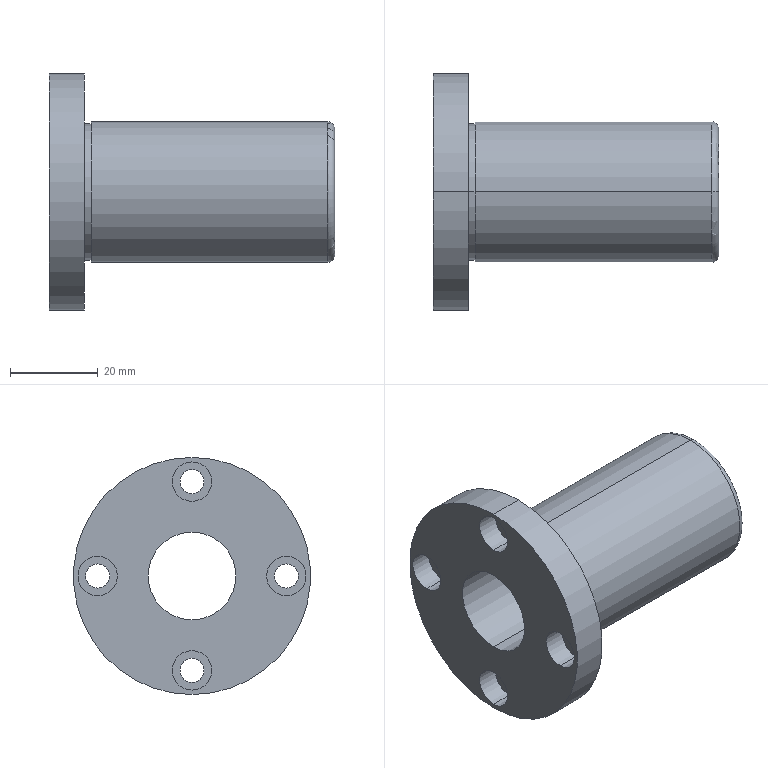Part | SolidWorks | features LPattern 1, RevCut 1, Revolution 1 | 1 solid | 34 faces | box 65 x 54 x 54 mm | volume 42042 mm3 | cylinder 24 | plane 8 | torus 2 | commonest cylinder face diameters 5.5 x8 9 x8 20 x2 31 x2 32 x2 54 x2
STEP:
#1=CARTESIAN_POINT('',(8.,-21.5,-2.75));
#2=VERTEX_POINT('',#1);
#3=CARTESIAN_POINT('',(8.,-21.5,2.75));
#4=VERTEX_POINT('',#3);
#5=CARTESIAN_POINT('',(8.,-21.5,0.));
#6=DIRECTION('',(-1.,0.,0.));
#7=DIRECTION('',(0.,0.,1.));
#8=AXIS2_PLACEMENT_3D('',#5,#6,#7);
#9=CIRCLE('',#8,2.75);
#10=EDGE_CURVE('',#2,#4,#9,.T.);
#11=ORIENTED_EDGE('',*,*,#10,.F.);
#12=CARTESIAN_POINT('',(5.1,-21.5,-2.75));
#13=VERTEX_POINT('',#12);
#14=CARTESIAN_POINT('',(8.,-21.5,-2.75));
#15=DIRECTION('',(-1.,0.,0.));
#16=VECTOR('',#15,1000.);
#17=LINE('',#14,#16);
#18=EDGE_CURVE('',#2,#13,#17,.T.);
#19=ORIENTED_EDGE('',*,*,#18,.T.);
#20=CARTESIAN_POINT('',(5.1,-21.5,2.75));
#21=VERTEX_POINT('',#20);
#22=CARTESIAN_POINT('',(5.1,-21.5,0.));
#23=DIRECTION('',(-1.,0.,0.));
#24=DIRECTION('',(0.,0.,1.));
#25=AXIS2_PLACEMENT_3D('',#22,#23,#24);
#26=CIRCLE('',#25,2.75);
#27=EDGE_CURVE('',#13,#21,#26,.T.);
#28=ORIENTED_EDGE('',*,*,#27,.T.);
#29=CARTESIAN_POINT('',(8.,-21.5,2.75));
#30=DIRECTION('',(-1.,0.,0.));
#31=VECTOR('',#30,1000.);
#32=LINE('',#29,#31);
#33=EDGE_CURVE('',#4,#21,#32,.T.);
#34=ORIENTED_EDGE('',*,*,#33,.F.);
#35=EDGE_LOOP('',(#11,#19,#28,#34));
#36=FACE_OUTER_BOUND('',#35,.T.);
#37=CARTESIAN_POINT('',(8.,-21.5,0.));
#38=DIRECTION('',(-1.,0.,0.));
#39=DIRECTION('',(0.,0.,1.));
#40=AXIS2_PLACEMENT_3D('',#37,#38,#39);
#41=CYLINDRICAL_SURFACE('',#40,2.75);
#42=ADVANCED_FACE('',(#36),#41,.F.);
#43=CARTESIAN_POINT('',(5.1,-21.5,-4.5));
#44=VERTEX_POINT('',#43);
#45=CARTESIAN_POINT('',(5.1,-21.5,4.5));
#46=VERTEX_POINT('',#45);
#47=CARTESIAN_POINT('',(5.1,-21.5,0.));
#48=DIRECTION('',(-1.,0.,0.));
#49=DIRECTION('',(0.,0.,1.));
#50=AXIS2_PLACEMENT_3D('',#47,#48,#49);
#51=CIRCLE('',#50,4.5);
#52=EDGE_CURVE('',#44,#46,#51,.T.);
#53=ORIENTED_EDGE('',*,*,#52,.F.);
#54=CARTESIAN_POINT('',(0.,-21.5,-4.5));
#55=VERTEX_POINT('',#54);
#56=CARTESIAN_POINT('',(8.,-21.5,-4.5));
#57=DIRECTION('',(-1.,0.,0.));
#58=VECTOR('',#57,1000.);
#59=LINE('',#56,#58);
#60=EDGE_CURVE('',#44,#55,#59,.T.);
#61=ORIENTED_EDGE('',*,*,#60,.T.);
#62=CARTESIAN_POINT('',(0.,-21.5,4.5));
#63=VERTEX_POINT('',#62);
#64=CARTESIAN_POINT('',(0.,-21.5,0.));
#65=DIRECTION('',(-1.,0.,0.));
#66=DIRECTION('',(0.,0.,1.));
#67=AXIS2_PLACEMENT_3D('',#64,#65,#66);
#68=CIRCLE('',#67,4.5);
#69=EDGE_CURVE('',#55,#63,#68,.T.);
#70=ORIENTED_EDGE('',*,*,#69,.T.);
#71=CARTESIAN_POINT('',(8.,-21.5,4.5));
#72=DIRECTION('',(-1.,0.,0.));
#73=VECTOR('',#72,1000.);
#74=LINE('',#71,#73);
#75=EDGE_CURVE('',#46,#63,#74,.T.);
#76=ORIENTED_EDGE('',*,*,#75,.F.);
#77=EDGE_LOOP('',(#53,#61,#70,#76));
#78=FACE_OUTER_BOUND('',#77,.T.);
#79=CARTESIAN_POINT('',(8.,-21.5,0.));
#80=DIRECTION('',(-1.,0.,0.));
#81=DIRECTION('',(0.,0.,1.));
#82=AXIS2_PLACEMENT_3D('',#79,#80,#81);
#83=CYLINDRICAL_SURFACE('',#82,4.5);
#84=ADVANCED_FACE('',(#78),#83,.F.);
#85=CARTESIAN_POINT('',(8.,0.,18.75));
#86=VERTEX_POINT('',#85);
#87=CARTESIAN_POINT('',(8.,0.,24.25));
#88=VERTEX_POINT('',#87);
#89=CARTESIAN_POINT('',(8.,0.,21.5));
#90=DIRECTION('',(-1.,0.,0.));
#91=DIRECTION('',(0.,0.,1.));
#92=AXIS2_PLACEMENT_3D('',#89,#90,#91);
#93=CIRCLE('',#92,2.75);
#94=EDGE_CURVE('',#86,#88,#93,.T.);
#95=ORIENTED_EDGE('',*,*,#94,.F.);
#96=CARTESIAN_POINT('',(5.1,0.,18.75));
#97=VERTEX_POINT('',#96);
#98=CARTESIAN_POINT('',(8.,0.,18.75));
#99=DIRECTION('',(-1.,0.,0.));
#100=VECTOR('',#99,1000.);
#101=LINE('',#98,#100);
#102=EDGE_CURVE('',#86,#97,#101,.T.);
#103=ORIENTED_EDGE('',*,*,#102,.T.);
#104=CARTESIAN_POINT('',(5.1,0.,24.25));
#105=VERTEX_POINT('',#104);
#106=CARTESIAN_POINT('',(5.1,0.,21.5));
#107=DIRECTION('',(-1.,0.,0.));
#108=DIRECTION('',(0.,0.,1.));
#109=AXIS2_PLACEMENT_3D('',#106,#107,#108);
#110=CIRCLE('',#109,2.75);
#111=EDGE_CURVE('',#97,#105,#110,.T.);
#112=ORIENTED_EDGE('',*,*,#111,.T.);
#113=CARTESIAN_POINT('',(8.,0.,24.25));
#114=DIRECTION('',(-1.,0.,0.));
#115=VECTOR('',#114,1000.);
#116=LINE('',#113,#115);
#117=EDGE_CURVE('',#88,#105,#116,.T.);
#118=ORIENTED_EDGE('',*,*,#117,.F.);
#119=EDGE_LOOP('',(#95,#103,#112,#118));
#120=FACE_OUTER_BOUND('',#119,.T.);
#121=CARTESIAN_POINT('',(8.,0.,21.5));
#122=DIRECTION('',(-1.,0.,0.));
#123=DIRECTION('',(0.,0.,1.));
#124=AXIS2_PLACEMENT_3D('',#121,#122,#123);
#125=CYLINDRICAL_SURFACE('',#124,2.75);
#126=ADVANCED_FACE('',(#120),#125,.F.);
#127=CARTESIAN_POINT('',(5.1,0.,17.));
#128=VERTEX_POINT('',#127);
#129=CARTESIAN_POINT('',(5.1,0.,26.));
#130=VERTEX_POINT('',#129);
#131=CARTESIAN_POINT('',(5.1,0.,21.5));
#132=DIRECTION('',(-1.,0.,0.));
#133=DIRECTION('',(0.,0.,1.));
#134=AXIS2_PLACEMENT_3D('',#131,#132,#133);
#135=CIRCLE('',#134,4.5);
#136=EDGE_CURVE('',#128,#130,#135,.T.);
#137=ORIENTED_EDGE('',*,*,#136,.F.);
#138=CARTESIAN_POINT('',(0.,0.,17.));
#139=VERTEX_POINT('',#138);
#140=CARTESIAN_POINT('',(8.,0.,17.));
#141=DIRECTION('',(-1.,0.,0.));
#142=VECTOR('',#141,1000.);
#143=LINE('',#140,#142);
#144=EDGE_CURVE('',#128,#139,#143,.T.);
#145=ORIENTED_EDGE('',*,*,#144,.T.);
#146=CARTESIAN_POINT('',(0.,0.,26.));
#147=VERTEX_POINT('',#146);
#148=CARTESIAN_POINT('',(0.,0.,21.5));
#149=DIRECTION('',(-1.,0.,0.));
#150=DIRECTION('',(0.,0.,1.));
#151=AXIS2_PLACEMENT_3D('',#148,#149,#150);
#152=CIRCLE('',#151,4.5);
#153=EDGE_CURVE('',#139,#147,#152,.T.);
#154=ORIENTED_EDGE('',*,*,#153,.T.);
#155=CARTESIAN_POINT('',(8.,0.,26.));
#156=DIRECTION('',(-1.,0.,0.));
#157=VECTOR('',#156,1000.);
#158=LINE('',#155,#157);
#159=EDGE_CURVE('',#130,#147,#158,.T.);
#160=ORIENTED_EDGE('',*,*,#159,.F.);
#161=EDGE_LOOP('',(#137,#145,#154,#160));
#162=FACE_OUTER_BOUND('',#161,.T.);
#163=CARTESIAN_POINT('',(8.,0.,21.5));
#164=DIRECTION('',(-1.,0.,0.));
#165=DIRECTION('',(0.,0.,1.));
#166=AXIS2_PLACEMENT_3D('',#163,#164,#165);
#167=CYLINDRICAL_SURFACE('',#166,4.5);
#168=ADVANCED_FACE('',(#162),#167,.F.);
#169=CARTESIAN_POINT('',(8.,0.,-24.25));
#170=VERTEX_POINT('',#169);
#171=CARTESIAN_POINT('',(8.,0.,-18.75));
#172=VERTEX_POINT('',#171);
#173=CARTESIAN_POINT('',(8.,0.,-21.5));
#174=DIRECTION('',(-1.,0.,0.));
#175=DIRECTION('',(0.,0.,1.));
#176=AXIS2_PLACEMENT_3D('',#173,#174,#175);
#177=CIRCLE('',#176,2.75);
#178=EDGE_CURVE('',#170,#172,#177,.T.);
#179=ORIENTED_EDGE('',*,*,#178,.F.);
#180=CARTESIAN_POINT('',(5.1,0.,-24.25));
#181=VERTEX_POINT('',#180);
#182=CARTESIAN_POINT('',(8.,0.,-24.25));
#183=DIRECTION('',(-1.,0.,0.));
#184=VECTOR('',#183,1000.);
#185=LINE('',#182,#184);
#186=EDGE_CURVE('',#170,#181,#185,.T.);
#187=ORIENTED_EDGE('',*,*,#186,.T.);
#188=CARTESIAN_POINT('',(5.1,0.,-18.75));
#189=VERTEX_POINT('',#188);
#190=CARTESIAN_POINT('',(5.1,0.,-21.5));
#191=DIRECTION('',(-1.,0.,0.));
#192=DIRECTION('',(0.,0.,1.));
#193=AXIS2_PLACEMENT_3D('',#190,#191,#192);
#194=CIRCLE('',#193,2.75);
#195=EDGE_CURVE('',#181,#189,#194,.T.);
#196=ORIENTED_EDGE('',*,*,#195,.T.);
#197=CARTESIAN_POINT('',(8.,0.,-18.75));
#198=DIRECTION('',(-1.,0.,0.));
#199=VECTOR('',#198,1000.);
#200=LINE('',#197,#199);
#201=EDGE_CURVE('',#172,#189,#200,.T.);
#202=ORIENTED_EDGE('',*,*,#201,.F.);
#203=EDGE_LOOP('',(#179,#187,#196,#202));
#204=FACE_OUTER_BOUND('',#203,.T.);
#205=CARTESIAN_POINT('',(8.,0.,-21.5));
#206=DIRECTION('',(-1.,0.,0.));
#207=DIRECTION('',(0.,0.,1.));
#208=AXIS2_PLACEMENT_3D('',#205,#206,#207);
#209=CYLINDRICAL_SURFACE('',#208,2.75);
#210=ADVANCED_FACE('',(#204),#209,.F.);
#211=CARTESIAN_POINT('',(5.1,0.,-26.));
#212=VERTEX_POINT('',#211);
#213=CARTESIAN_POINT('',(5.1,0.,-17.));
#214=VERTEX_POINT('',#213);
#215=CARTESIAN_POINT('',(5.1,0.,-21.5));
#216=DIRECTION('',(-1.,0.,0.));
#217=DIRECTION('',(0.,0.,1.));
#218=AXIS2_PLACEMENT_3D('',#215,#216,#217);
#219=CIRCLE('',#218,4.5);
#220=EDGE_CURVE('',#212,#214,#219,.T.);
#221=ORIENTED_EDGE('',*,*,#220,.F.);
#222=CARTESIAN_POINT('',(0.,0.,-26.));
#223=VERTEX_POINT('',#222);
#224=CARTESIAN_POINT('',(8.,0.,-26.));
#225=DIRECTION('',(-1.,0.,0.));
#226=VECTOR('',#225,1000.);
#227=LINE('',#224,#226);
#228=EDGE_CURVE('',#212,#223,#227,.T.);
#229=ORIENTED_EDGE('',*,*,#228,.T.);
#230=CARTESIAN_POINT('',(0.,0.,-17.));
#231=VERTEX_POINT('',#230);
#232=CARTESIAN_POINT('',(0.,0.,-21.5));
#233=DIRECTION('',(-1.,0.,0.));
#234=DIRECTION('',(0.,0.,1.));
#235=AXIS2_PLACEMENT_3D('',#232,#233,#234);
#236=CIRCLE('',#235,4.5);
#237=EDGE_CURVE('',#223,#231,#236,.T.);
#238=ORIENTED_EDGE('',*,*,#237,.T.);
#239=CARTESIAN_POINT('',(8.,0.,-17.));
#240=DIRECTION('',(-1.,0.,0.));
#241=VECTOR('',#240,1000.);
#242=LINE('',#239,#241);
#243=EDGE_CURVE('',#214,#231,#242,.T.);
#244=ORIENTED_EDGE('',*,*,#243,.F.);
#245=EDGE_LOOP('',(#221,#229,#238,#244));
#246=FACE_OUTER_BOUND('',#245,.T.);
#247=CARTESIAN_POINT('',(8.,0.,-21.5));
#248=DIRECTION('',(-1.,0.,0.));
#249=DIRECTION('',(0.,0.,1.));
#250=AXIS2_PLACEMENT_3D('',#247,#248,#249);
#251=CYLINDRICAL_SURFACE('',#250,4.5);
#252=ADVANCED_FACE('',(#246),#251,.F.);
#253=CARTESIAN_POINT('',(8.,21.5,-2.75));
#254=VERTEX_POINT('',#253);
#255=CARTESIAN_POINT('',(8.,21.5,2.75));
#256=VERTEX_POINT('',#255);
#257=CARTESIAN_POINT('',(8.,21.5,0.));
#258=DIRECTION('',(-1.,0.,0.));
#259=DIRECTION('',(0.,0.,1.));
#260=AXIS2_PLACEMENT_3D('',#257,#258,#259);
#261=CIRCLE('',#260,2.75);
#262=EDGE_CURVE('',#254,#256,#261,.T.);
#263=ORIENTED_EDGE('',*,*,#262,.F.);
#264=CARTESIAN_POINT('',(5.1,21.5,-2.75));
#265=VERTEX_POINT('',#264);
#266=CARTESIAN_POINT('',(8.,21.5,-2.75));
#267=DIRECTION('',(-1.,0.,0.));
#268=VECTOR('',#267,1000.);
#269=LINE('',#266,#268);
#270=EDGE_CURVE('',#254,#265,#269,.T.);
#271=ORIENTED_EDGE('',*,*,#270,.T.);
#272=CARTESIAN_POINT('',(5.1,21.5,2.75));
#273=VERTEX_POINT('',#272);
#274=CARTESIAN_POINT('',(5.1,21.5,0.));
#275=DIRECTION('',(-1.,0.,0.));
#276=DIRECTION('',(0.,0.,1.));
#277=AXIS2_PLACEMENT_3D('',#274,#275,#276);
#278=CIRCLE('',#277,2.75);
#279=EDGE_CURVE('',#265,#273,#278,.T.);
#280=ORIENTED_EDGE('',*,*,#279,.T.);
#281=CARTESIAN_POINT('',(8.,21.5,2.75));
#282=DIRECTION('',(-1.,0.,0.));
#283=VECTOR('',#282,1000.);
#284=LINE('',#281,#283);
#285=EDGE_CURVE('',#256,#273,#284,.T.);
#286=ORIENTED_EDGE('',*,*,#285,.F.);
#287=EDGE_LOOP('',(#263,#271,#280,#286));
#288=FACE_OUTER_BOUND('',#287,.T.);
#289=CARTESIAN_POINT('',(8.,21.5,0.));
#290=DIRECTION('',(-1.,0.,0.));
#291=DIRECTION('',(0.,0.,1.));
#292=AXIS2_PLACEMENT_3D('',#289,#290,#291);
#293=CYLINDRICAL_SURFACE('',#292,2.75);
#294=ADVANCED_FACE('',(#288),#293,.F.);
#295=CARTESIAN_POINT('',(5.1,21.5,-4.5));
#296=VERTEX_POINT('',#295);
#297=CARTESIAN_POINT('',(5.1,21.5,4.5));
#298=VERTEX_POINT('',#297);
#299=CARTESIAN_POINT('',(5.1,21.5,0.));
#300=DIRECTION('',(-1.,0.,0.));
#301=DIRECTION('',(0.,0.,1.));
#302=AXIS2_PLACEMENT_3D('',#299,#300,#301);
#303=CIRCLE('',#302,4.5);
#304=EDGE_CURVE('',#296,#298,#303,.T.);
#305=ORIENTED_EDGE('',*,*,#304,.F.);
#306=CARTESIAN_POINT('',(0.,21.5,-4.5));
#307=VERTEX_POINT('',#306);
#308=CARTESIAN_POINT('',(8.,21.5,-4.5));
#309=DIRECTION('',(-1.,0.,0.));
#310=VECTOR('',#309,1000.);
#311=LINE('',#308,#310);
#312=EDGE_CURVE('',#296,#307,#311,.T.);
#313=ORIENTED_EDGE('',*,*,#312,.T.);
#314=CARTESIAN_POINT('',(0.,21.5,4.5));
#315=VERTEX_POINT('',#314);
#316=CARTESIAN_POINT('',(0.,21.5,0.));
#317=DIRECTION('',(-1.,0.,0.));
#318=DIRECTION('',(0.,0.,1.));
#319=AXIS2_PLACEMENT_3D('',#316,#317,#318);
#320=CIRCLE('',#319,4.5);
#321=EDGE_CURVE('',#307,#315,#320,.T.);
#322=ORIENTED_EDGE('',*,*,#321,.T.);
#323=CARTESIAN_POINT('',(8.,21.5,4.5));
#324=DIRECTION('',(-1.,0.,0.));
#325=VECTOR('',#324,1000.);
#326=LINE('',#323,#325);
#327=EDGE_CURVE('',#298,#315,#326,.T.);
#328=ORIENTED_EDGE('',*,*,#327,.F.);
#329=EDGE_LOOP('',(#305,#313,#322,#328));
#330=FACE_OUTER_BOUND('',#329,.T.);
#331=CARTESIAN_POINT('',(8.,21.5,0.));
#332=DIRECTION('',(-1.,0.,0.));
#333=DIRECTION('',(0.,0.,1.));
#334=AXIS2_PLACEMENT_3D('',#331,#332,#333);
#335=CYLINDRICAL_SURFACE('',#334,4.5);
#336=ADVANCED_FACE('',(#330),#335,.F.);
#337=CARTESIAN_POINT('',(9.5,0.,15.5));
#338=VERTEX_POINT('',#337);
#339=CARTESIAN_POINT('',(9.5,0.,-15.5));
#340=VERTEX_POINT('',#339);
#341=CARTESIAN_POINT('',(9.5,0.,0.));
#342=DIRECTION('',(-1.,0.,0.));
#343=DIRECTION('',(0.,0.,1.));
#344=AXIS2_PLACEMENT_3D('',#341,#342,#343);
#345=CIRCLE('',#344,15.5);
#346=EDGE_CURVE('',#338,#340,#345,.T.);
#347=ORIENTED_EDGE('',*,*,#346,.T.);
#348=CARTESIAN_POINT('',(8.,0.,-15.5));
#349=VERTEX_POINT('',#348);
#350=CARTESIAN_POINT('',(65.,0.,-15.5));
#351=DIRECTION('',(-1.,0.,0.));
#352=VECTOR('',#351,1000.);
#353=LINE('',#350,#352);
#354=EDGE_CURVE('',#340,#349,#353,.T.);
#355=ORIENTED_EDGE('',*,*,#354,.T.);
#356=CARTESIAN_POINT('',(8.,0.,15.5));
#357=VERTEX_POINT('',#356);
#358=CARTESIAN_POINT('',(8.,0.,0.));
#359=DIRECTION('',(-1.,0.,0.));
#360=DIRECTION('',(0.,0.,1.));
#361=AXIS2_PLACEMENT_3D('',#358,#359,#360);
#362=CIRCLE('',#361,15.5);
#363=EDGE_CURVE('',#357,#349,#362,.T.);
#364=ORIENTED_EDGE('',*,*,#363,.F.);
#365=CARTESIAN_POINT('',(65.,0.,15.5));
#366=DIRECTION('',(-1.,0.,0.));
#367=VECTOR('',#366,1000.);
#368=LINE('',#365,#367);
#369=EDGE_CURVE('',#338,#357,#368,.T.);
#370=ORIENTED_EDGE('',*,*,#369,.F.);
#371=EDGE_LOOP('',(#347,#355,#364,#370));
#372=FACE_OUTER_BOUND('',#371,.T.);
#373=CARTESIAN_POINT('',(65.,0.,0.));
#374=DIRECTION('',(-1.,0.,0.));
#375=DIRECTION('',(0.,0.,1.));
#376=AXIS2_PLACEMENT_3D('',#373,#374,#375);
#377=CYLINDRICAL_SURFACE('',#376,15.5);
#378=ADVANCED_FACE('',(#372),#377,.T.);
#379=CARTESIAN_POINT('',(63.4,0.,16.));
#380=VERTEX_POINT('',#379);
#381=CARTESIAN_POINT('',(63.4,0.,-16.));
#382=VERTEX_POINT('',#381);
#383=CARTESIAN_POINT('',(63.4,0.,0.));
#384=DIRECTION('',(-1.,0.,0.));
#385=DIRECTION('',(0.,0.,1.));
#386=AXIS2_PLACEMENT_3D('',#383,#384,#385);
#387=CIRCLE('',#386,16.);
#388=EDGE_CURVE('',#380,#382,#387,.T.);
#389=ORIENTED_EDGE('',*,*,#388,.T.);
#390=CARTESIAN_POINT('',(9.5,0.,-16.));
#391=VERTEX_POINT('',#390);
#392=CARTESIAN_POINT('',(65.,0.,-16.));
#393=DIRECTION('',(-1.,0.,0.));
#394=VECTOR('',#393,1000.);
#395=LINE('',#392,#394);
#396=EDGE_CURVE('',#382,#391,#395,.T.);
#397=ORIENTED_EDGE('',*,*,#396,.T.);
#398=CARTESIAN_POINT('',(9.5,0.,16.));
#399=VERTEX_POINT('',#398);
#400=CARTESIAN_POINT('',(9.5,0.,0.));
#401=DIRECTION('',(-1.,0.,0.));
#402=DIRECTION('',(0.,0.,1.));
#403=AXIS2_PLACEMENT_3D('',#400,#401,#402);
#404=CIRCLE('',#403,16.);
#405=EDGE_CURVE('',#399,#391,#404,.T.);
#406=ORIENTED_EDGE('',*,*,#405,.F.);
#407=CARTESIAN_POINT('',(65.,0.,16.));
#408=DIRECTION('',(-1.,0.,0.));
#409=VECTOR('',#408,1000.);
#410=LINE('',#407,#409);
#411=EDGE_CURVE('',#380,#399,#410,.T.);
#412=ORIENTED_EDGE('',*,*,#411,.F.);
#413=EDGE_LOOP('',(#389,#397,#406,#412));
#414=FACE_OUTER_BOUND('',#413,.T.);
#415=CARTESIAN_POINT('',(65.,0.,0.));
#416=DIRECTION('',(-1.,0.,0.));
#417=DIRECTION('',(0.,0.,1.));
#418=AXIS2_PLACEMENT_3D('',#415,#416,#417);
#419=CYLINDRICAL_SURFACE('',#418,16.);
#420=ADVANCED_FACE('',(#414),#419,.T.);
#421=CARTESIAN_POINT('',(65.,0.,14.4));
#422=VERTEX_POINT('',#421);
#423=CARTESIAN_POINT('',(65.,0.,-14.4));
#424=VERTEX_POINT('',#423);
#425=CARTESIAN_POINT('',(65.,0.,0.));
#426=DIRECTION('',(-1.,0.,0.));
#427=DIRECTION('',(0.,0.,1.));
#428=AXIS2_PLACEMENT_3D('',#425,#426,#427);
#429=CIRCLE('',#428,14.4);
#430=EDGE_CURVE('',#422,#424,#429,.T.);
#431=ORIENTED_EDGE('',*,*,#430,.T.);
#432=CARTESIAN_POINT('',(63.4,0.,-14.4));
#433=DIRECTION('',(0.,1.,0.));
#434=DIRECTION('',(0.,0.,1.));
#435=AXIS2_PLACEMENT_3D('',#432,#433,#434);
#436=CIRCLE('',#435,1.6);
#437=EDGE_CURVE('',#424,#382,#436,.T.);
#438=ORIENTED_EDGE('',*,*,#437,.T.);
#439=ORIENTED_EDGE('',*,*,#388,.F.);
#440=CARTESIAN_POINT('',(63.4,0.,14.4));
#441=DIRECTION('',(0.,-1.,0.));
#442=DIRECTION('',(0.,0.,-1.));
#443=AXIS2_PLACEMENT_3D('',#440,#441,#442);
#444=CIRCLE('',#443,1.6);
#445=EDGE_CURVE('',#422,#380,#444,.T.);
#446=ORIENTED_EDGE('',*,*,#445,.F.);
#447=EDGE_LOOP('',(#431,#438,#439,#446));
#448=FACE_OUTER_BOUND('',#447,.T.);
#449=CARTESIAN_POINT('',(63.4,0.,0.));
#450=DIRECTION('',(-1.,0.,0.));
#451=DIRECTION('',(0.,0.,1.));
#452=AXIS2_PLACEMENT_3D('',#449,#450,#451);
#453=TOROIDAL_SURFACE('',#452,14.4,1.6);
#454=ADVANCED_FACE('',(#448),#453,.T.);
#455=CARTESIAN_POINT('',(65.,0.,-10.));
#456=VERTEX_POINT('',#455);
#457=CARTESIAN_POINT('',(65.,0.,10.));
#458=VERTEX_POINT('',#457);
#459=CARTESIAN_POINT('',(65.,0.,0.));
#460=DIRECTION('',(-1.,0.,0.));
#461=DIRECTION('',(0.,0.,1.));
#462=AXIS2_PLACEMENT_3D('',#459,#460,#461);
#463=CIRCLE('',#462,10.);
#464=EDGE_CURVE('',#456,#458,#463,.T.);
#465=ORIENTED_EDGE('',*,*,#464,.F.);
#466=CARTESIAN_POINT('',(0.,0.,-10.));
#467=VERTEX_POINT('',#466);
#468=CARTESIAN_POINT('',(65.,0.,-10.));
#469=DIRECTION('',(-1.,0.,0.));
#470=VECTOR('',#469,1000.);
#471=LINE('',#468,#470);
#472=EDGE_CURVE('',#456,#467,#471,.T.);
#473=ORIENTED_EDGE('',*,*,#472,.T.);
#474=CARTESIAN_POINT('',(0.,0.,10.));
#475=VERTEX_POINT('',#474);
#476=CARTESIAN_POINT('',(0.,0.,0.));
#477=DIRECTION('',(-1.,0.,0.));
#478=DIRECTION('',(0.,0.,1.));
#479=AXIS2_PLACEMENT_3D('',#476,#477,#478);
#480=CIRCLE('',#479,10.);
#481=EDGE_CURVE('',#467,#475,#480,.T.);
#482=ORIENTED_EDGE('',*,*,#481,.T.);
#483=CARTESIAN_POINT('',(65.,0.,10.));
#484=DIRECTION('',(-1.,0.,0.));
#485=VECTOR('',#484,1000.);
#486=LINE('',#483,#485);
#487=EDGE_CURVE('',#458,#475,#486,.T.);
#488=ORIENTED_EDGE('',*,*,#487,.F.);
#489=EDGE_LOOP('',(#465,#473,#482,#488));
#490=FACE_OUTER_BOUND('',#489,.T.);
#491=CARTESIAN_POINT('',(65.,0.,0.));
#492=DIRECTION('',(-1.,0.,0.));
#493=DIRECTION('',(0.,0.,1.));
#494=AXIS2_PLACEMENT_3D('',#491,#492,#493);
#495=CYLINDRICAL_SURFACE('',#494,10.);
#496=ADVANCED_FACE('',(#490),#495,.F.);
#497=CARTESIAN_POINT('',(8.,0.,27.));
#498=VERTEX_POINT('',#497);
#499=CARTESIAN_POINT('',(8.,0.,-27.));
#500=VERTEX_POINT('',#499);
#501=CARTESIAN_POINT('',(8.,0.,0.));
#502=DIRECTION('',(-1.,0.,0.));
#503=DIRECTION('',(0.,0.,1.));
#504=AXIS2_PLACEMENT_3D('',#501,#502,#503);
#505=CIRCLE('',#504,27.);
#506=EDGE_CURVE('',#498,#500,#505,.T.);
#507=ORIENTED_EDGE('',*,*,#506,.T.);
#508=CARTESIAN_POINT('',(0.,0.,-27.));
#509=VERTEX_POINT('',#508);
#510=CARTESIAN_POINT('',(65.,0.,-27.));
#511=DIRECTION('',(-1.,0.,0.));
#512=VECTOR('',#511,1000.);
#513=LINE('',#510,#512);
#514=EDGE_CURVE('',#500,#509,#513,.T.);
#515=ORIENTED_EDGE('',*,*,#514,.T.);
#516=CARTESIAN_POINT('',(0.,0.,27.));
#517=VERTEX_POINT('',#516);
#518=CARTESIAN_POINT('',(0.,0.,0.));
#519=DIRECTION('',(-1.,0.,0.));
#520=DIRECTION('',(0.,0.,1.));
#521=AXIS2_PLACEMENT_3D('',#518,#519,#520);
#522=CIRCLE('',#521,27.);
#523=EDGE_CURVE('',#517,#509,#522,.T.);
#524=ORIENTED_EDGE('',*,*,#523,.F.);
#525=CARTESIAN_POINT('',(65.,0.,27.));
#526=DIRECTION('',(-1.,0.,0.));
#527=VECTOR('',#526,1000.);
#528=LINE('',#525,#527);
#529=EDGE_CURVE('',#498,#517,#528,.T.);
#530=ORIENTED_EDGE('',*,*,#529,.F.);
#531=EDGE_LOOP('',(#507,#515,#524,#530));
#532=FACE_OUTER_BOUND('',#531,.T.);
#533=CARTESIAN_POINT('',(65.,0.,0.));
#534=DIRECTION('',(-1.,0.,0.));
#535=DIRECTION('',(0.,0.,1.));
#536=AXIS2_PLACEMENT_3D('',#533,#534,#535);
#537=CYLINDRICAL_SURFACE('',#536,27.);
#538=ADVANCED_FACE('',(#532),#537,.T.);
#539=CARTESIAN_POINT('',(0.,0.,21.5));
#540=DIRECTION('',(-1.,0.,0.));
#541=DIRECTION('',(0.,0.,1.));
#542=AXIS2_PLACEMENT_3D('',#539,#540,#541);
#543=CIRCLE('',#542,4.5);
#544=EDGE_CURVE('',#147,#139,#543,.T.);
#545=ORIENTED_EDGE('',*,*,#544,.F.);
#546=ORIENTED_EDGE('',*,*,#153,.F.);
#547=EDGE_LOOP('',(#545,#546));
#548=FACE_BOUND('',#547,.T.);
#549=CARTESIAN_POINT('',(0.,21.5,0.));
#550=DIRECTION('',(-1.,0.,0.));
#551=DIRECTION('',(0.,0.,1.));
#552=AXIS2_PLACEMENT_3D('',#549,#550,#551);
#553=CIRCLE('',#552,4.5);
#554=EDGE_CURVE('',#315,#307,#553,.T.);
#555=ORIENTED_EDGE('',*,*,#554,.F.);
#556=ORIENTED_EDGE('',*,*,#321,.F.);
#557=EDGE_LOOP('',(#555,#556));
#558=FACE_BOUND('',#557,.T.);
#559=CARTESIAN_POINT('',(0.,0.,0.));
#560=DIRECTION('',(-1.,0.,0.));
#561=DIRECTION('',(0.,0.,1.));
#562=AXIS2_PLACEMENT_3D('',#559,#560,#561);
#563=CIRCLE('',#562,10.);
#564=EDGE_CURVE('',#475,#467,#563,.T.);
#565=ORIENTED_EDGE('',*,*,#564,.F.);
#566=ORIENTED_EDGE('',*,*,#481,.F.);
#567=EDGE_LOOP('',(#565,#566));
#568=FACE_BOUND('',#567,.T.);
#569=ORIENTED_EDGE('',*,*,#523,.T.);
#570=CARTESIAN_POINT('',(0.,0.,0.));
#571=DIRECTION('',(-1.,0.,0.));
#572=DIRECTION('',(0.,0.,1.));
#573=AXIS2_PLACEMENT_3D('',#570,#571,#572);
#574=CIRCLE('',#573,27.);
#575=EDGE_CURVE('',#509,#517,#574,.T.);
#576=ORIENTED_EDGE('',*,*,#575,.T.);
#577=EDGE_LOOP('',(#569,#576));
#578=FACE_OUTER_BOUND('',#577,.T.);
#579=CARTESIAN_POINT('',(0.,0.,-21.5));
#580=DIRECTION('',(-1.,0.,0.));
#581=DIRECTION('',(0.,0.,1.));
#582=AXIS2_PLACEMENT_3D('',#579,#580,#581);
#583=CIRCLE('',#582,4.5);
#584=EDGE_CURVE('',#231,#223,#583,.T.);
#585=ORIENTED_EDGE('',*,*,#584,.F.);
#586=ORIENTED_EDGE('',*,*,#237,.F.);
#587=EDGE_LOOP('',(#585,#586));
#588=FACE_BOUND('',#587,.T.);
#589=CARTESIAN_POINT('',(0.,-21.5,0.));
#590=DIRECTION('',(-1.,0.,0.));
#591=DIRECTION('',(0.,0.,1.));
#592=AXIS2_PLACEMENT_3D('',#589,#590,#591);
#593=CIRCLE('',#592,4.5);
#594=EDGE_CURVE('',#63,#55,#593,.T.);
#595=ORIENTED_EDGE('',*,*,#594,.F.);
#596=ORIENTED_EDGE('',*,*,#69,.F.);
#597=EDGE_LOOP('',(#595,#596));
#598=FACE_BOUND('',#597,.T.);
#599=CARTESIAN_POINT('',(0.,27.,0.));
#600=DIRECTION('',(1.,0.,0.));
#601=DIRECTION('',(0.,0.,-1.));
#602=AXIS2_PLACEMENT_3D('',#599,#600,#601);
#603=PLANE('',#602);
#604=ADVANCED_FACE('',(#548,#558,#568,#578,#588,#598),#603,.F.);
#605=CARTESIAN_POINT('',(8.,0.,21.5));
#606=DIRECTION('',(-1.,0.,0.));
#607=DIRECTION('',(0.,0.,1.));
#608=AXIS2_PLACEMENT_3D('',#605,#606,#607);
#609=CIRCLE('',#608,2.75);
#610=EDGE_CURVE('',#88,#86,#609,.T.);
#611=ORIENTED_EDGE('',*,*,#610,.T.);
#612=ORIENTED_EDGE('',*,*,#94,.T.);
#613=EDGE_LOOP('',(#611,#612));
#614=FACE_BOUND('',#613,.T.);
#615=CARTESIAN_POINT('',(8.,21.5,0.));
#616=DIRECTION('',(-1.,0.,0.));
#617=DIRECTION('',(0.,0.,1.));
#618=AXIS2_PLACEMENT_3D('',#615,#616,#617);
#619=CIRCLE('',#618,2.75);
#620=EDGE_CURVE('',#256,#254,#619,.T.);
#621=ORIENTED_EDGE('',*,*,#620,.T.);
#622=ORIENTED_EDGE('',*,*,#262,.T.);
#623=EDGE_LOOP('',(#621,#622));
#624=FACE_BOUND('',#623,.T.);
#625=ORIENTED_EDGE('',*,*,#506,.F.);
#626=CARTESIAN_POINT('',(8.,0.,0.));
#627=DIRECTION('',(-1.,0.,0.));
#628=DIRECTION('',(0.,0.,1.));
#629=AXIS2_PLACEMENT_3D('',#626,#627,#628);
#630=CIRCLE('',#629,27.);
#631=EDGE_CURVE('',#500,#498,#630,.T.);
#632=ORIENTED_EDGE('',*,*,#631,.F.);
#633=EDGE_LOOP('',(#625,#632));
#634=FACE_OUTER_BOUND('',#633,.T.);
#635=ORIENTED_EDGE('',*,*,#363,.T.);
#636=CARTESIAN_POINT('',(8.,0.,0.));
#637=DIRECTION('',(-1.,0.,0.));
#638=DIRECTION('',(0.,0.,1.));
#639=AXIS2_PLACEMENT_3D('',#636,#637,#638);
#640=CIRCLE('',#639,15.5);
#641=EDGE_CURVE('',#349,#357,#640,.T.);
#642=ORIENTED_EDGE('',*,*,#641,.T.);
#643=EDGE_LOOP('',(#635,#642));
#644=FACE_BOUND('',#643,.T.);
#645=CARTESIAN_POINT('',(8.,0.,-21.5));
#646=DIRECTION('',(-1.,0.,0.));
#647=DIRECTION('',(0.,0.,1.));
#648=AXIS2_PLACEMENT_3D('',#645,#646,#647);
#649=CIRCLE('',#648,2.75);
#650=EDGE_CURVE('',#172,#170,#649,.T.);
#651=ORIENTED_EDGE('',*,*,#650,.T.);
#652=ORIENTED_EDGE('',*,*,#178,.T.);
#653=EDGE_LOOP('',(#651,#652));
#654=FACE_BOUND('',#653,.T.);
#655=CARTESIAN_POINT('',(8.,-21.5,0.));
#656=DIRECTION('',(-1.,0.,0.));
#657=DIRECTION('',(0.,0.,1.));
#658=AXIS2_PLACEMENT_3D('',#655,#656,#657);
#659=CIRCLE('',#658,2.75);
#660=EDGE_CURVE('',#4,#2,#659,.T.);
#661=ORIENTED_EDGE('',*,*,#660,.T.);
#662=ORIENTED_EDGE('',*,*,#10,.T.);
#663=EDGE_LOOP('',(#661,#662));
#664=FACE_BOUND('',#663,.T.);
#665=CARTESIAN_POINT('',(8.,15.5,0.));
#666=DIRECTION('',(-1.,0.,0.));
#667=DIRECTION('',(0.,0.,1.));
#668=AXIS2_PLACEMENT_3D('',#665,#666,#667);
#669=PLANE('',#668);
#670=ADVANCED_FACE('',(#614,#624,#634,#644,#654,#664),#669,.F.);
#671=ORIENTED_EDGE('',*,*,#514,.F.);
#672=ORIENTED_EDGE('',*,*,#631,.T.);
#673=ORIENTED_EDGE('',*,*,#529,.T.);
#674=ORIENTED_EDGE('',*,*,#575,.F.);
#675=EDGE_LOOP('',(#671,#672,#673,#674));
#676=FACE_OUTER_BOUND('',#675,.T.);
#677=CARTESIAN_POINT('',(65.,0.,0.));
#678=DIRECTION('',(-1.,0.,0.));
#679=DIRECTION('',(0.,0.,1.));
#680=AXIS2_PLACEMENT_3D('',#677,#678,#679);
#681=CYLINDRICAL_SURFACE('',#680,27.);
#682=ADVANCED_FACE('',(#676),#681,.T.);
#683=ORIENTED_EDGE('',*,*,#472,.F.);
#684=CARTESIAN_POINT('',(65.,0.,0.));
#685=DIRECTION('',(-1.,0.,0.));
#686=DIRECTION('',(0.,0.,1.));
#687=AXIS2_PLACEMENT_3D('',#684,#685,#686);
#688=CIRCLE('',#687,10.);
#689=EDGE_CURVE('',#458,#456,#688,.T.);
#690=ORIENTED_EDGE('',*,*,#689,.F.);
#691=ORIENTED_EDGE('',*,*,#487,.T.);
#692=ORIENTED_EDGE('',*,*,#564,.T.);
#693=EDGE_LOOP('',(#683,#690,#691,#692));
#694=FACE_OUTER_BOUND('',#693,.T.);
#695=CARTESIAN_POINT('',(65.,0.,0.));
#696=DIRECTION('',(-1.,0.,0.));
#697=DIRECTION('',(0.,0.,1.));
#698=AXIS2_PLACEMENT_3D('',#695,#696,#697);
#699=CYLINDRICAL_SURFACE('',#698,10.);
#700=ADVANCED_FACE('',(#694),#699,.F.);
#701=ORIENTED_EDGE('',*,*,#430,.F.);
#702=CARTESIAN_POINT('',(65.,0.,0.));
#703=DIRECTION('',(-1.,0.,0.));
#704=DIRECTION('',(0.,0.,1.));
#705=AXIS2_PLACEMENT_3D('',#702,#703,#704);
#706=CIRCLE('',#705,14.4);
#707=EDGE_CURVE('',#424,#422,#706,.T.);
#708=ORIENTED_EDGE('',*,*,#707,.F.);
#709=EDGE_LOOP('',(#701,#708));
#710=FACE_OUTER_BOUND('',#709,.T.);
#711=ORIENTED_EDGE('',*,*,#689,.T.);
#712=ORIENTED_EDGE('',*,*,#464,.T.);
#713=EDGE_LOOP('',(#711,#712));
#714=FACE_BOUND('',#713,.T.);
#715=CARTESIAN_POINT('',(65.,10.,0.));
#716=DIRECTION('',(-1.,0.,0.));
#717=DIRECTION('',(0.,0.,1.));
#718=AXIS2_PLACEMENT_3D('',#715,#716,#717);
#719=PLANE('',#718);
#720=ADVANCED_FACE('',(#710,#714),#719,.F.);
#721=ORIENTED_EDGE('',*,*,#437,.F.);
#722=ORIENTED_EDGE('',*,*,#707,.T.);
#723=ORIENTED_EDGE('',*,*,#445,.T.);
#724=CARTESIAN_POINT('',(63.4,0.,0.));
#725=DIRECTION('',(-1.,0.,0.));
#726=DIRECTION('',(0.,0.,1.));
#727=AXIS2_PLACEMENT_3D('',#724,#725,#726);
#728=CIRCLE('',#727,16.);
#729=EDGE_CURVE('',#382,#380,#728,.T.);
#730=ORIENTED_EDGE('',*,*,#729,.F.);
#731=EDGE_LOOP('',(#721,#722,#723,#730));
#732=FACE_OUTER_BOUND('',#731,.T.);
#733=CARTESIAN_POINT('',(63.4,0.,0.));
#734=DIRECTION('',(-1.,0.,0.));
#735=DIRECTION('',(0.,0.,1.));
#736=AXIS2_PLACEMENT_3D('',#733,#734,#735);
#737=TOROIDAL_SURFACE('',#736,14.4,1.6);
#738=ADVANCED_FACE('',(#732),#737,.T.);
#739=ORIENTED_EDGE('',*,*,#396,.F.);
#740=ORIENTED_EDGE('',*,*,#729,.T.);
#741=ORIENTED_EDGE('',*,*,#411,.T.);
#742=CARTESIAN_POINT('',(9.5,0.,0.));
#743=DIRECTION('',(-1.,0.,0.));
#744=DIRECTION('',(0.,0.,1.));
#745=AXIS2_PLACEMENT_3D('',#742,#743,#744);
#746=CIRCLE('',#745,16.);
#747=EDGE_CURVE('',#391,#399,#746,.T.);
#748=ORIENTED_EDGE('',*,*,#747,.F.);
#749=EDGE_LOOP('',(#739,#740,#741,#748));
#750=FACE_OUTER_BOUND('',#749,.T.);
#751=CARTESIAN_POINT('',(65.,0.,0.));
#752=DIRECTION('',(-1.,0.,0.));
#753=DIRECTION('',(0.,0.,1.));
#754=AXIS2_PLACEMENT_3D('',#751,#752,#753);
#755=CYLINDRICAL_SURFACE('',#754,16.);
#756=ADVANCED_FACE('',(#750),#755,.T.);
#757=ORIENTED_EDGE('',*,*,#346,.F.);
#758=CARTESIAN_POINT('',(9.5,0.,0.));
#759=DIRECTION('',(-1.,0.,0.));
#760=DIRECTION('',(0.,0.,1.));
#761=AXIS2_PLACEMENT_3D('',#758,#759,#760);
#762=CIRCLE('',#761,15.5);
#763=EDGE_CURVE('',#340,#338,#762,.T.);
#764=ORIENTED_EDGE('',*,*,#763,.F.);
#765=EDGE_LOOP('',(#757,#764));
#766=FACE_BOUND('',#765,.T.);
#767=ORIENTED_EDGE('',*,*,#405,.T.);
#768=ORIENTED_EDGE('',*,*,#747,.T.);
#769=EDGE_LOOP('',(#767,#768));
#770=FACE_OUTER_BOUND('',#769,.T.);
#771=CARTESIAN_POINT('',(9.5,16.,0.));
#772=DIRECTION('',(1.,0.,0.));
#773=DIRECTION('',(0.,0.,-1.));
#774=AXIS2_PLACEMENT_3D('',#771,#772,#773);
#775=PLANE('',#774);
#776=ADVANCED_FACE('',(#766,#770),#775,.F.);
#777=ORIENTED_EDGE('',*,*,#354,.F.);
#778=ORIENTED_EDGE('',*,*,#763,.T.);
#779=ORIENTED_EDGE('',*,*,#369,.T.);
#780=ORIENTED_EDGE('',*,*,#641,.F.);
#781=EDGE_LOOP('',(#777,#778,#779,#780));
#782=FACE_OUTER_BOUND('',#781,.T.);
#783=CARTESIAN_POINT('',(65.,0.,0.));
#784=DIRECTION('',(-1.,0.,0.));
#785=DIRECTION('',(0.,0.,1.));
#786=AXIS2_PLACEMENT_3D('',#783,#784,#785);
#787=CYLINDRICAL_SURFACE('',#786,15.5);
#788=ADVANCED_FACE('',(#782),#787,.T.);
#789=ORIENTED_EDGE('',*,*,#312,.F.);
#790=CARTESIAN_POINT('',(5.1,21.5,0.));
#791=DIRECTION('',(-1.,0.,0.));
#792=DIRECTION('',(0.,0.,1.));
#793=AXIS2_PLACEMENT_3D('',#790,#791,#792);
#794=CIRCLE('',#793,4.5);
#795=EDGE_CURVE('',#298,#296,#794,.T.);
#796=ORIENTED_EDGE('',*,*,#795,.F.);
#797=ORIENTED_EDGE('',*,*,#327,.T.);
#798=ORIENTED_EDGE('',*,*,#554,.T.);
#799=EDGE_LOOP('',(#789,#796,#797,#798));
#800=FACE_OUTER_BOUND('',#799,.T.);
#801=CARTESIAN_POINT('',(8.,21.5,0.));
#802=DIRECTION('',(-1.,0.,0.));
#803=DIRECTION('',(0.,0.,1.));
#804=AXIS2_PLACEMENT_3D('',#801,#802,#803);
#805=CYLINDRICAL_SURFACE('',#804,4.5);
#806=ADVANCED_FACE('',(#800),#805,.F.);
#807=ORIENTED_EDGE('',*,*,#795,.T.);
#808=ORIENTED_EDGE('',*,*,#304,.T.);
#809=EDGE_LOOP('',(#807,#808));
#810=FACE_OUTER_BOUND('',#809,.T.);
#811=CARTESIAN_POINT('',(5.1,21.5,0.));
#812=DIRECTION('',(-1.,0.,0.));
#813=DIRECTION('',(0.,0.,1.));
#814=AXIS2_PLACEMENT_3D('',#811,#812,#813);
#815=CIRCLE('',#814,2.75);
#816=EDGE_CURVE('',#273,#265,#815,.T.);
#817=ORIENTED_EDGE('',*,*,#816,.F.);
#818=ORIENTED_EDGE('',*,*,#279,.F.);
#819=EDGE_LOOP('',(#817,#818));
#820=FACE_BOUND('',#819,.T.);
#821=CARTESIAN_POINT('',(5.1,26.,0.));
#822=DIRECTION('',(-1.,0.,0.));
#823=DIRECTION('',(0.,0.,1.));
#824=AXIS2_PLACEMENT_3D('',#821,#822,#823);
#825=PLANE('',#824);
#826=ADVANCED_FACE('',(#810,#820),#825,.T.);
#827=ORIENTED_EDGE('',*,*,#270,.F.);
#828=ORIENTED_EDGE('',*,*,#620,.F.);
#829=ORIENTED_EDGE('',*,*,#285,.T.);
#830=ORIENTED_EDGE('',*,*,#816,.T.);
#831=EDGE_LOOP('',(#827,#828,#829,#830));
#832=FACE_OUTER_BOUND('',#831,.T.);
#833=CARTESIAN_POINT('',(8.,21.5,0.));
#834=DIRECTION('',(-1.,0.,0.));
#835=DIRECTION('',(0.,0.,1.));
#836=AXIS2_PLACEMENT_3D('',#833,#834,#835);
#837=CYLINDRICAL_SURFACE('',#836,2.75);
#838=ADVANCED_FACE('',(#832),#837,.F.);
#839=ORIENTED_EDGE('',*,*,#228,.F.);
#840=CARTESIAN_POINT('',(5.1,0.,-21.5));
#841=DIRECTION('',(-1.,0.,0.));
#842=DIRECTION('',(0.,0.,1.));
#843=AXIS2_PLACEMENT_3D('',#840,#841,#842);
#844=CIRCLE('',#843,4.5);
#845=EDGE_CURVE('',#214,#212,#844,.T.);
#846=ORIENTED_EDGE('',*,*,#845,.F.);
#847=ORIENTED_EDGE('',*,*,#243,.T.);
#848=ORIENTED_EDGE('',*,*,#584,.T.);
#849=EDGE_LOOP('',(#839,#846,#847,#848));
#850=FACE_OUTER_BOUND('',#849,.T.);
#851=CARTESIAN_POINT('',(8.,0.,-21.5));
#852=DIRECTION('',(-1.,0.,0.));
#853=DIRECTION('',(0.,0.,1.));
#854=AXIS2_PLACEMENT_3D('',#851,#852,#853);
#855=CYLINDRICAL_SURFACE('',#854,4.5);
#856=ADVANCED_FACE('',(#850),#855,.F.);
#857=ORIENTED_EDGE('',*,*,#845,.T.);
#858=ORIENTED_EDGE('',*,*,#220,.T.);
#859=EDGE_LOOP('',(#857,#858));
#860=FACE_OUTER_BOUND('',#859,.T.);
#861=CARTESIAN_POINT('',(5.1,0.,-21.5));
#862=DIRECTION('',(-1.,0.,0.));
#863=DIRECTION('',(0.,0.,1.));
#864=AXIS2_PLACEMENT_3D('',#861,#862,#863);
#865=CIRCLE('',#864,2.75);
#866=EDGE_CURVE('',#189,#181,#865,.T.);
#867=ORIENTED_EDGE('',*,*,#866,.F.);
#868=ORIENTED_EDGE('',*,*,#195,.F.);
#869=EDGE_LOOP('',(#867,#868));
#870=FACE_BOUND('',#869,.T.);
#871=CARTESIAN_POINT('',(5.1,4.5,-21.5));
#872=DIRECTION('',(-1.,0.,0.));
#873=DIRECTION('',(0.,0.,1.));
#874=AXIS2_PLACEMENT_3D('',#871,#872,#873);
#875=PLANE('',#874);
#876=ADVANCED_FACE('',(#860,#870),#875,.T.);
#877=ORIENTED_EDGE('',*,*,#186,.F.);
#878=ORIENTED_EDGE('',*,*,#650,.F.);
#879=ORIENTED_EDGE('',*,*,#201,.T.);
#880=ORIENTED_EDGE('',*,*,#866,.T.);
#881=EDGE_LOOP('',(#877,#878,#879,#880));
#882=FACE_OUTER_BOUND('',#881,.T.);
#883=CARTESIAN_POINT('',(8.,0.,-21.5));
#884=DIRECTION('',(-1.,0.,0.));
#885=DIRECTION('',(0.,0.,1.));
#886=AXIS2_PLACEMENT_3D('',#883,#884,#885);
#887=CYLINDRICAL_SURFACE('',#886,2.75);
#888=ADVANCED_FACE('',(#882),#887,.F.);
#889=ORIENTED_EDGE('',*,*,#144,.F.);
#890=CARTESIAN_POINT('',(5.1,0.,21.5));
#891=DIRECTION('',(-1.,0.,0.));
#892=DIRECTION('',(0.,0.,1.));
#893=AXIS2_PLACEMENT_3D('',#890,#891,#892);
#894=CIRCLE('',#893,4.5);
#895=EDGE_CURVE('',#130,#128,#894,.T.);
#896=ORIENTED_EDGE('',*,*,#895,.F.);
#897=ORIENTED_EDGE('',*,*,#159,.T.);
#898=ORIENTED_EDGE('',*,*,#544,.T.);
#899=EDGE_LOOP('',(#889,#896,#897,#898));
#900=FACE_OUTER_BOUND('',#899,.T.);
#901=CARTESIAN_POINT('',(8.,0.,21.5));
#902=DIRECTION('',(-1.,0.,0.));
#903=DIRECTION('',(0.,0.,1.));
#904=AXIS2_PLACEMENT_3D('',#901,#902,#903);
#905=CYLINDRICAL_SURFACE('',#904,4.5);
#906=ADVANCED_FACE('',(#900),#905,.F.);
#907=ORIENTED_EDGE('',*,*,#895,.T.);
#908=ORIENTED_EDGE('',*,*,#136,.T.);
#909=EDGE_LOOP('',(#907,#908));
#910=FACE_OUTER_BOUND('',#909,.T.);
#911=CARTESIAN_POINT('',(5.1,0.,21.5));
#912=DIRECTION('',(-1.,0.,0.));
#913=DIRECTION('',(0.,0.,1.));
#914=AXIS2_PLACEMENT_3D('',#911,#912,#913);
#915=CIRCLE('',#914,2.75);
#916=EDGE_CURVE('',#105,#97,#915,.T.);
#917=ORIENTED_EDGE('',*,*,#916,.F.);
#918=ORIENTED_EDGE('',*,*,#111,.F.);
#919=EDGE_LOOP('',(#917,#918));
#920=FACE_BOUND('',#919,.T.);
#921=CARTESIAN_POINT('',(5.1,4.5,21.5));
#922=DIRECTION('',(-1.,0.,0.));
#923=DIRECTION('',(0.,0.,1.));
#924=AXIS2_PLACEMENT_3D('',#921,#922,#923);
#925=PLANE('',#924);
#926=ADVANCED_FACE('',(#910,#920),#925,.T.);
#927=ORIENTED_EDGE('',*,*,#102,.F.);
#928=ORIENTED_EDGE('',*,*,#610,.F.);
#929=ORIENTED_EDGE('',*,*,#117,.T.);
#930=ORIENTED_EDGE('',*,*,#916,.T.);
#931=EDGE_LOOP('',(#927,#928,#929,#930));
#932=FACE_OUTER_BOUND('',#931,.T.);
#933=CARTESIAN_POINT('',(8.,0.,21.5));
#934=DIRECTION('',(-1.,0.,0.));
#935=DIRECTION('',(0.,0.,1.));
#936=AXIS2_PLACEMENT_3D('',#933,#934,#935);
#937=CYLINDRICAL_SURFACE('',#936,2.75);
#938=ADVANCED_FACE('',(#932),#937,.F.);
#939=ORIENTED_EDGE('',*,*,#60,.F.);
#940=CARTESIAN_POINT('',(5.1,-21.5,0.));
#941=DIRECTION('',(-1.,0.,0.));
#942=DIRECTION('',(0.,0.,1.));
#943=AXIS2_PLACEMENT_3D('',#940,#941,#942);
#944=CIRCLE('',#943,4.5);
#945=EDGE_CURVE('',#46,#44,#944,.T.);
#946=ORIENTED_EDGE('',*,*,#945,.F.);
#947=ORIENTED_EDGE('',*,*,#75,.T.);
#948=ORIENTED_EDGE('',*,*,#594,.T.);
#949=EDGE_LOOP('',(#939,#946,#947,#948));
#950=FACE_OUTER_BOUND('',#949,.T.);
#951=CARTESIAN_POINT('',(8.,-21.5,0.));
#952=DIRECTION('',(-1.,0.,0.));
#953=DIRECTION('',(0.,0.,1.));
#954=AXIS2_PLACEMENT_3D('',#951,#952,#953);
#955=CYLINDRICAL_SURFACE('',#954,4.5);
#956=ADVANCED_FACE('',(#950),#955,.F.);
#957=ORIENTED_EDGE('',*,*,#945,.T.);
#958=ORIENTED_EDGE('',*,*,#52,.T.);
#959=EDGE_LOOP('',(#957,#958));
#960=FACE_OUTER_BOUND('',#959,.T.);
#961=CARTESIAN_POINT('',(5.1,-21.5,0.));
#962=DIRECTION('',(-1.,0.,0.));
#963=DIRECTION('',(0.,0.,1.));
#964=AXIS2_PLACEMENT_3D('',#961,#962,#963);
#965=CIRCLE('',#964,2.75);
#966=EDGE_CURVE('',#21,#13,#965,.T.);
#967=ORIENTED_EDGE('',*,*,#966,.F.);
#968=ORIENTED_EDGE('',*,*,#27,.F.);
#969=EDGE_LOOP('',(#967,#968));
#970=FACE_BOUND('',#969,.T.);
#971=CARTESIAN_POINT('',(5.1,-17.,0.));
#972=DIRECTION('',(-1.,0.,0.));
#973=DIRECTION('',(0.,0.,1.));
#974=AXIS2_PLACEMENT_3D('',#971,#972,#973);
#975=PLANE('',#974);
#976=ADVANCED_FACE('',(#960,#970),#975,.T.);
#977=ORIENTED_EDGE('',*,*,#18,.F.);
#978=ORIENTED_EDGE('',*,*,#660,.F.);
#979=ORIENTED_EDGE('',*,*,#33,.T.);
#980=ORIENTED_EDGE('',*,*,#966,.T.);
#981=EDGE_LOOP('',(#977,#978,#979,#980));
#982=FACE_OUTER_BOUND('',#981,.T.);
#983=CARTESIAN_POINT('',(8.,-21.5,0.));
#984=DIRECTION('',(-1.,0.,0.));
#985=DIRECTION('',(0.,0.,1.));
#986=AXIS2_PLACEMENT_3D('',#983,#984,#985);
#987=CYLINDRICAL_SURFACE('',#986,2.75);
#988=ADVANCED_FACE('',(#982),#987,.F.);
#989=CLOSED_SHELL('',(#42,#84,#126,#168,#210,#252,#294,#336,#378,#420,#454,#496,#538,#604,#670,#682,#700,#720,#738,#756,#776,#788,#806,#826,#838,#856,#876,#888,#906,#926,#938,#956,#976,#988));
#990=MANIFOLD_SOLID_BREP('',#989);
#991=CARTESIAN_POINT('',(0.,0.,0.));
#992=DIRECTION('',(0.,0.,1.));
#993=DIRECTION('',(1.,0.,0.));
#994=AXIS2_PLACEMENT_3D('',#991,#992,#993);
#995=(LENGTH_UNIT()NAMED_UNIT(*)SI_UNIT(.MILLI.,.METRE.));
#996=UNCERTAINTY_MEASURE_WITH_UNIT(LENGTH_MEASURE(0.00001),#995,'','');
#997=(NAMED_UNIT(*)PLANE_ANGLE_UNIT()SI_UNIT($,.RADIAN.));
#998=(NAMED_UNIT(*)SI_UNIT($,.STERADIAN.)SOLID_ANGLE_UNIT());
#999=(GEOMETRIC_REPRESENTATION_CONTEXT(3)GLOBAL_UNCERTAINTY_ASSIGNED_CONTEXT((#996))GLOBAL_UNIT_ASSIGNED_CONTEXT((#995,#997,#998))REPRESENTATION_CONTEXT('',''));
#1000=ADVANCED_BREP_SHAPE_REPRESENTATION('',(#990,#994),#999);